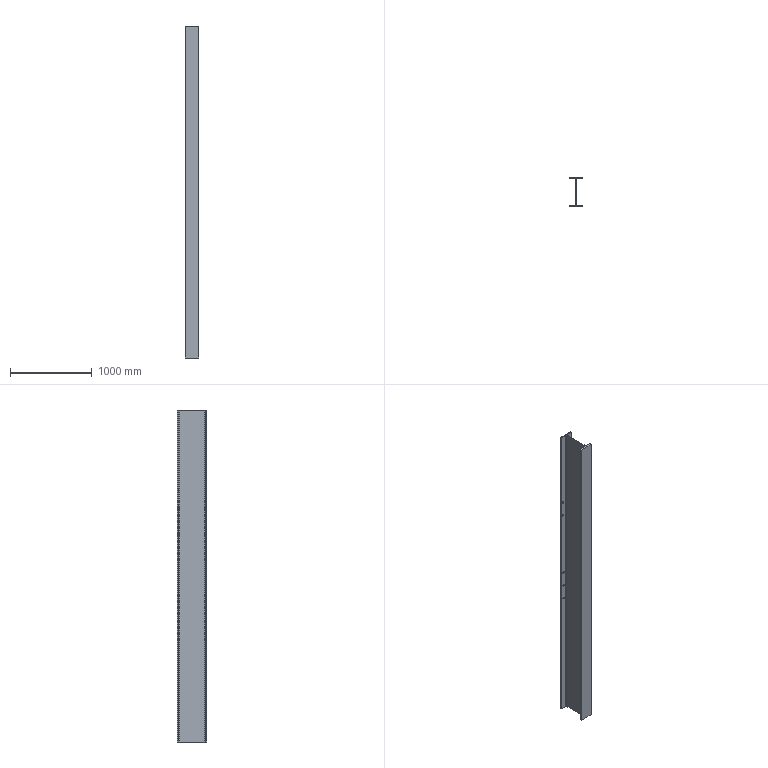Part | SolidWorks | features Chamfer 1, Extrusion 1, ICE 1, SketchHole 1 | 1 solid | 39 faces | box 171.323 x 355.092 x 4064 mm | volume 26304101 mm3 | cylinder 24 | plane 15 | commonest cylinder face diameters 20.574 x20 25.4 x4
STEP:
#1=CARTESIAN_POINT('',(61.087,165.989,1644.65));
#2=VERTEX_POINT('',#1);
#3=CARTESIAN_POINT('',(40.513,165.989,1644.65));
#4=VERTEX_POINT('',#3);
#5=CARTESIAN_POINT('',(50.8,165.989,1644.65));
#6=DIRECTION('',(0.,1.,0.));
#7=DIRECTION('',(-1.,0.,0.));
#8=AXIS2_PLACEMENT_3D('',#5,#6,#7);
#9=CIRCLE('',#8,10.287);
#10=EDGE_CURVE('',#2,#4,#9,.T.);
#11=ORIENTED_EDGE('',*,*,#10,.F.);
#12=CARTESIAN_POINT('',(61.087,177.546,1644.65));
#13=VERTEX_POINT('',#12);
#14=CARTESIAN_POINT('',(61.087,157.546,1644.65));
#15=DIRECTION('',(0.,1.,0.));
#16=VECTOR('',#15,1000.);
#17=LINE('',#14,#16);
#18=EDGE_CURVE('',#2,#13,#17,.T.);
#19=ORIENTED_EDGE('',*,*,#18,.T.);
#20=CARTESIAN_POINT('',(40.513,177.546,1644.65));
#21=VERTEX_POINT('',#20);
#22=CARTESIAN_POINT('',(50.8,177.546,1644.65));
#23=DIRECTION('',(0.,1.,0.));
#24=DIRECTION('',(-1.,0.,0.));
#25=AXIS2_PLACEMENT_3D('',#22,#23,#24);
#26=CIRCLE('',#25,10.287);
#27=EDGE_CURVE('',#13,#21,#26,.T.);
#28=ORIENTED_EDGE('',*,*,#27,.T.);
#29=CARTESIAN_POINT('',(40.513,157.546,1644.65));
#30=DIRECTION('',(0.,1.,0.));
#31=VECTOR('',#30,1000.);
#32=LINE('',#29,#31);
#33=EDGE_CURVE('',#4,#21,#32,.T.);
#34=ORIENTED_EDGE('',*,*,#33,.F.);
#35=EDGE_LOOP('',(#11,#19,#28,#34));
#36=FACE_OUTER_BOUND('',#35,.T.);
#37=CARTESIAN_POINT('',(50.8,157.546,1644.65));
#38=DIRECTION('',(0.,1.,0.));
#39=DIRECTION('',(-1.,0.,0.));
#40=AXIS2_PLACEMENT_3D('',#37,#38,#39);
#41=CYLINDRICAL_SURFACE('',#40,10.287);
#42=ADVANCED_FACE('',(#36),#41,.F.);
#43=CARTESIAN_POINT('',(61.087,165.989,1835.15));
#44=VERTEX_POINT('',#43);
#45=CARTESIAN_POINT('',(40.513,165.989,1835.15));
#46=VERTEX_POINT('',#45);
#47=CARTESIAN_POINT('',(50.8,165.989,1835.15));
#48=DIRECTION('',(0.,1.,0.));
#49=DIRECTION('',(-1.,0.,0.));
#50=AXIS2_PLACEMENT_3D('',#47,#48,#49);
#51=CIRCLE('',#50,10.287);
#52=EDGE_CURVE('',#44,#46,#51,.T.);
#53=ORIENTED_EDGE('',*,*,#52,.F.);
#54=CARTESIAN_POINT('',(61.087,177.546,1835.15));
#55=VERTEX_POINT('',#54);
#56=CARTESIAN_POINT('',(61.087,157.546,1835.15));
#57=DIRECTION('',(0.,1.,0.));
#58=VECTOR('',#57,1000.);
#59=LINE('',#56,#58);
#60=EDGE_CURVE('',#44,#55,#59,.T.);
#61=ORIENTED_EDGE('',*,*,#60,.T.);
#62=CARTESIAN_POINT('',(40.513,177.546,1835.15));
#63=VERTEX_POINT('',#62);
#64=CARTESIAN_POINT('',(50.8,177.546,1835.15));
#65=DIRECTION('',(0.,1.,0.));
#66=DIRECTION('',(-1.,0.,0.));
#67=AXIS2_PLACEMENT_3D('',#64,#65,#66);
#68=CIRCLE('',#67,10.287);
#69=EDGE_CURVE('',#55,#63,#68,.T.);
#70=ORIENTED_EDGE('',*,*,#69,.T.);
#71=CARTESIAN_POINT('',(40.513,157.546,1835.15));
#72=DIRECTION('',(0.,1.,0.));
#73=VECTOR('',#72,1000.);
#74=LINE('',#71,#73);
#75=EDGE_CURVE('',#46,#63,#74,.T.);
#76=ORIENTED_EDGE('',*,*,#75,.F.);
#77=EDGE_LOOP('',(#53,#61,#70,#76));
#78=FACE_OUTER_BOUND('',#77,.T.);
#79=CARTESIAN_POINT('',(50.8,157.546,1835.15));
#80=DIRECTION('',(0.,1.,0.));
#81=DIRECTION('',(-1.,0.,0.));
#82=AXIS2_PLACEMENT_3D('',#79,#80,#81);
#83=CYLINDRICAL_SURFACE('',#82,10.287);
#84=ADVANCED_FACE('',(#78),#83,.F.);
#85=CARTESIAN_POINT('',(-40.513,165.989,1644.65));
#86=VERTEX_POINT('',#85);
#87=CARTESIAN_POINT('',(-61.087,165.989,1644.65));
#88=VERTEX_POINT('',#87);
#89=CARTESIAN_POINT('',(-50.8,165.989,1644.65));
#90=DIRECTION('',(0.,1.,0.));
#91=DIRECTION('',(0.,0.,1.));
#92=AXIS2_PLACEMENT_3D('',#89,#90,#91);
#93=CIRCLE('',#92,10.287);
#94=EDGE_CURVE('',#86,#88,#93,.T.);
#95=ORIENTED_EDGE('',*,*,#94,.F.);
#96=CARTESIAN_POINT('',(-40.513,177.546,1644.65));
#97=VERTEX_POINT('',#96);
#98=CARTESIAN_POINT('',(-40.513,157.546,1644.65));
#99=DIRECTION('',(0.,1.,0.));
#100=VECTOR('',#99,1000.);
#101=LINE('',#98,#100);
#102=EDGE_CURVE('',#86,#97,#101,.T.);
#103=ORIENTED_EDGE('',*,*,#102,.T.);
#104=CARTESIAN_POINT('',(-61.087,177.546,1644.65));
#105=VERTEX_POINT('',#104);
#106=CARTESIAN_POINT('',(-50.8,177.546,1644.65));
#107=DIRECTION('',(0.,1.,0.));
#108=DIRECTION('',(-1.,0.,0.));
#109=AXIS2_PLACEMENT_3D('',#106,#107,#108);
#110=CIRCLE('',#109,10.287);
#111=EDGE_CURVE('',#97,#105,#110,.T.);
#112=ORIENTED_EDGE('',*,*,#111,.T.);
#113=CARTESIAN_POINT('',(-61.087,157.546,1644.65));
#114=DIRECTION('',(0.,1.,0.));
#115=VECTOR('',#114,1000.);
#116=LINE('',#113,#115);
#117=EDGE_CURVE('',#88,#105,#116,.T.);
#118=ORIENTED_EDGE('',*,*,#117,.F.);
#119=EDGE_LOOP('',(#95,#103,#112,#118));
#120=FACE_OUTER_BOUND('',#119,.T.);
#121=CARTESIAN_POINT('',(-50.8,157.546,1644.65));
#122=DIRECTION('',(0.,1.,0.));
#123=DIRECTION('',(-1.,0.,0.));
#124=AXIS2_PLACEMENT_3D('',#121,#122,#123);
#125=CYLINDRICAL_SURFACE('',#124,10.287);
#126=ADVANCED_FACE('',(#120),#125,.F.);
#127=CARTESIAN_POINT('',(-40.513,165.989,1835.15));
#128=VERTEX_POINT('',#127);
#129=CARTESIAN_POINT('',(-61.087,165.989,1835.15));
#130=VERTEX_POINT('',#129);
#131=CARTESIAN_POINT('',(-50.8,165.989,1835.15));
#132=DIRECTION('',(0.,1.,0.));
#133=DIRECTION('',(0.,0.,1.));
#134=AXIS2_PLACEMENT_3D('',#131,#132,#133);
#135=CIRCLE('',#134,10.287);
#136=EDGE_CURVE('',#128,#130,#135,.T.);
#137=ORIENTED_EDGE('',*,*,#136,.F.);
#138=CARTESIAN_POINT('',(-40.513,177.546,1835.15));
#139=VERTEX_POINT('',#138);
#140=CARTESIAN_POINT('',(-40.513,157.546,1835.15));
#141=DIRECTION('',(0.,1.,0.));
#142=VECTOR('',#141,1000.);
#143=LINE('',#140,#142);
#144=EDGE_CURVE('',#128,#139,#143,.T.);
#145=ORIENTED_EDGE('',*,*,#144,.T.);
#146=CARTESIAN_POINT('',(-61.087,177.546,1835.15));
#147=VERTEX_POINT('',#146);
#148=CARTESIAN_POINT('',(-50.8,177.546,1835.15));
#149=DIRECTION('',(0.,1.,0.));
#150=DIRECTION('',(-1.,0.,0.));
#151=AXIS2_PLACEMENT_3D('',#148,#149,#150);
#152=CIRCLE('',#151,10.287);
#153=EDGE_CURVE('',#139,#147,#152,.T.);
#154=ORIENTED_EDGE('',*,*,#153,.T.);
#155=CARTESIAN_POINT('',(-61.087,157.546,1835.15));
#156=DIRECTION('',(0.,1.,0.));
#157=VECTOR('',#156,1000.);
#158=LINE('',#155,#157);
#159=EDGE_CURVE('',#130,#147,#158,.T.);
#160=ORIENTED_EDGE('',*,*,#159,.F.);
#161=EDGE_LOOP('',(#137,#145,#154,#160));
#162=FACE_OUTER_BOUND('',#161,.T.);
#163=CARTESIAN_POINT('',(-50.8,157.546,1835.15));
#164=DIRECTION('',(0.,1.,0.));
#165=DIRECTION('',(-1.,0.,0.));
#166=AXIS2_PLACEMENT_3D('',#163,#164,#165);
#167=CYLINDRICAL_SURFACE('',#166,10.287);
#168=ADVANCED_FACE('',(#162),#167,.F.);
#169=CARTESIAN_POINT('',(-40.513,165.989,2025.65));
#170=VERTEX_POINT('',#169);
#171=CARTESIAN_POINT('',(-61.087,165.989,2025.65));
#172=VERTEX_POINT('',#171);
#173=CARTESIAN_POINT('',(-50.8,165.989,2025.65));
#174=DIRECTION('',(0.,1.,0.));
#175=DIRECTION('',(0.,0.,1.));
#176=AXIS2_PLACEMENT_3D('',#173,#174,#175);
#177=CIRCLE('',#176,10.287);
#178=EDGE_CURVE('',#170,#172,#177,.T.);
#179=ORIENTED_EDGE('',*,*,#178,.F.);
#180=CARTESIAN_POINT('',(-40.513,177.546,2025.65));
#181=VERTEX_POINT('',#180);
#182=CARTESIAN_POINT('',(-40.513,157.546,2025.65));
#183=DIRECTION('',(0.,1.,0.));
#184=VECTOR('',#183,1000.);
#185=LINE('',#182,#184);
#186=EDGE_CURVE('',#170,#181,#185,.T.);
#187=ORIENTED_EDGE('',*,*,#186,.T.);
#188=CARTESIAN_POINT('',(-61.087,177.546,2025.65));
#189=VERTEX_POINT('',#188);
#190=CARTESIAN_POINT('',(-50.8,177.546,2025.65));
#191=DIRECTION('',(0.,1.,0.));
#192=DIRECTION('',(-1.,0.,0.));
#193=AXIS2_PLACEMENT_3D('',#190,#191,#192);
#194=CIRCLE('',#193,10.287);
#195=EDGE_CURVE('',#181,#189,#194,.T.);
#196=ORIENTED_EDGE('',*,*,#195,.T.);
#197=CARTESIAN_POINT('',(-61.087,157.546,2025.65));
#198=DIRECTION('',(0.,1.,0.));
#199=VECTOR('',#198,1000.);
#200=LINE('',#197,#199);
#201=EDGE_CURVE('',#172,#189,#200,.T.);
#202=ORIENTED_EDGE('',*,*,#201,.F.);
#203=EDGE_LOOP('',(#179,#187,#196,#202));
#204=FACE_OUTER_BOUND('',#203,.T.);
#205=CARTESIAN_POINT('',(-50.8,157.546,2025.65));
#206=DIRECTION('',(0.,1.,0.));
#207=DIRECTION('',(-1.,0.,0.));
#208=AXIS2_PLACEMENT_3D('',#205,#206,#207);
#209=CYLINDRICAL_SURFACE('',#208,10.287);
#210=ADVANCED_FACE('',(#204),#209,.F.);
#211=CARTESIAN_POINT('',(61.087,165.989,2025.65));
#212=VERTEX_POINT('',#211);
#213=CARTESIAN_POINT('',(40.513,165.989,2025.65));
#214=VERTEX_POINT('',#213);
#215=CARTESIAN_POINT('',(50.8,165.989,2025.65));
#216=DIRECTION('',(0.,1.,0.));
#217=DIRECTION('',(-1.,0.,0.));
#218=AXIS2_PLACEMENT_3D('',#215,#216,#217);
#219=CIRCLE('',#218,10.287);
#220=EDGE_CURVE('',#212,#214,#219,.T.);
#221=ORIENTED_EDGE('',*,*,#220,.F.);
#222=CARTESIAN_POINT('',(61.087,177.546,2025.65));
#223=VERTEX_POINT('',#222);
#224=CARTESIAN_POINT('',(61.087,157.546,2025.65));
#225=DIRECTION('',(0.,1.,0.));
#226=VECTOR('',#225,1000.);
#227=LINE('',#224,#226);
#228=EDGE_CURVE('',#212,#223,#227,.T.);
#229=ORIENTED_EDGE('',*,*,#228,.T.);
#230=CARTESIAN_POINT('',(40.513,177.546,2025.65));
#231=VERTEX_POINT('',#230);
#232=CARTESIAN_POINT('',(50.8,177.546,2025.65));
#233=DIRECTION('',(0.,1.,0.));
#234=DIRECTION('',(-1.,0.,0.));
#235=AXIS2_PLACEMENT_3D('',#232,#233,#234);
#236=CIRCLE('',#235,10.287);
#237=EDGE_CURVE('',#223,#231,#236,.T.);
#238=ORIENTED_EDGE('',*,*,#237,.T.);
#239=CARTESIAN_POINT('',(40.513,157.546,2025.65));
#240=DIRECTION('',(0.,1.,0.));
#241=VECTOR('',#240,1000.);
#242=LINE('',#239,#241);
#243=EDGE_CURVE('',#214,#231,#242,.T.);
#244=ORIENTED_EDGE('',*,*,#243,.F.);
#245=EDGE_LOOP('',(#221,#229,#238,#244));
#246=FACE_OUTER_BOUND('',#245,.T.);
#247=CARTESIAN_POINT('',(50.8,157.546,2025.65));
#248=DIRECTION('',(0.,1.,0.));
#249=DIRECTION('',(-1.,0.,0.));
#250=AXIS2_PLACEMENT_3D('',#247,#248,#249);
#251=CYLINDRICAL_SURFACE('',#250,10.287);
#252=ADVANCED_FACE('',(#246),#251,.F.);
#253=CARTESIAN_POINT('',(53.213,165.989,2889.25));
#254=VERTEX_POINT('',#253);
#255=CARTESIAN_POINT('',(73.787,165.989,2889.25));
#256=VERTEX_POINT('',#255);
#257=CARTESIAN_POINT('',(63.5,165.989,2889.25));
#258=DIRECTION('',(0.,-1.,0.));
#259=DIRECTION('',(-1.,0.,0.));
#260=AXIS2_PLACEMENT_3D('',#257,#258,#259);
#261=CIRCLE('',#260,10.287);
#262=EDGE_CURVE('',#254,#256,#261,.T.);
#263=ORIENTED_EDGE('',*,*,#262,.T.);
#264=CARTESIAN_POINT('',(73.787,177.546,2889.25));
#265=VERTEX_POINT('',#264);
#266=CARTESIAN_POINT('',(73.787,136.893,2889.25));
#267=DIRECTION('',(0.,1.,0.));
#268=VECTOR('',#267,1000.);
#269=LINE('',#266,#268);
#270=EDGE_CURVE('',#256,#265,#269,.T.);
#271=ORIENTED_EDGE('',*,*,#270,.T.);
#272=CARTESIAN_POINT('',(53.213,177.546,2889.25));
#273=VERTEX_POINT('',#272);
#274=CARTESIAN_POINT('',(63.5,177.546,2889.25));
#275=DIRECTION('',(0.,1.,0.));
#276=DIRECTION('',(-1.,0.,0.));
#277=AXIS2_PLACEMENT_3D('',#274,#275,#276);
#278=CIRCLE('',#277,10.287);
#279=EDGE_CURVE('',#265,#273,#278,.T.);
#280=ORIENTED_EDGE('',*,*,#279,.T.);
#281=CARTESIAN_POINT('',(53.213,136.893,2889.25));
#282=DIRECTION('',(0.,1.,0.));
#283=VECTOR('',#282,1000.);
#284=LINE('',#281,#283);
#285=EDGE_CURVE('',#254,#273,#284,.T.);
#286=ORIENTED_EDGE('',*,*,#285,.F.);
#287=EDGE_LOOP('',(#263,#271,#280,#286));
#288=FACE_OUTER_BOUND('',#287,.T.);
#289=CARTESIAN_POINT('',(63.5,136.893,2889.25));
#290=DIRECTION('',(0.,1.,0.));
#291=DIRECTION('',(-1.,0.,0.));
#292=AXIS2_PLACEMENT_3D('',#289,#290,#291);
#293=CYLINDRICAL_SURFACE('',#292,10.287);
#294=ADVANCED_FACE('',(#288),#293,.F.);
#295=CARTESIAN_POINT('',(-73.787,165.989,2889.25));
#296=VERTEX_POINT('',#295);
#297=CARTESIAN_POINT('',(-53.213,165.989,2889.25));
#298=VERTEX_POINT('',#297);
#299=CARTESIAN_POINT('',(-63.5,165.989,2889.25));
#300=DIRECTION('',(0.,-1.,0.));
#301=DIRECTION('',(-1.,0.,0.));
#302=AXIS2_PLACEMENT_3D('',#299,#300,#301);
#303=CIRCLE('',#302,10.287);
#304=EDGE_CURVE('',#296,#298,#303,.T.);
#305=ORIENTED_EDGE('',*,*,#304,.T.);
#306=CARTESIAN_POINT('',(-53.213,177.546,2889.25));
#307=VERTEX_POINT('',#306);
#308=CARTESIAN_POINT('',(-53.213,136.893,2889.25));
#309=DIRECTION('',(0.,1.,0.));
#310=VECTOR('',#309,1000.);
#311=LINE('',#308,#310);
#312=EDGE_CURVE('',#298,#307,#311,.T.);
#313=ORIENTED_EDGE('',*,*,#312,.T.);
#314=CARTESIAN_POINT('',(-73.787,177.546,2889.25));
#315=VERTEX_POINT('',#314);
#316=CARTESIAN_POINT('',(-63.5,177.546,2889.25));
#317=DIRECTION('',(0.,1.,0.));
#318=DIRECTION('',(-1.,0.,0.));
#319=AXIS2_PLACEMENT_3D('',#316,#317,#318);
#320=CIRCLE('',#319,10.287);
#321=EDGE_CURVE('',#307,#315,#320,.T.);
#322=ORIENTED_EDGE('',*,*,#321,.T.);
#323=CARTESIAN_POINT('',(-73.787,136.893,2889.25));
#324=DIRECTION('',(0.,1.,0.));
#325=VECTOR('',#324,1000.);
#326=LINE('',#323,#325);
#327=EDGE_CURVE('',#296,#315,#326,.T.);
#328=ORIENTED_EDGE('',*,*,#327,.F.);
#329=EDGE_LOOP('',(#305,#313,#322,#328));
#330=FACE_OUTER_BOUND('',#329,.T.);
#331=CARTESIAN_POINT('',(-63.5,136.893,2889.25));
#332=DIRECTION('',(0.,1.,0.));
#333=DIRECTION('',(-1.,0.,0.));
#334=AXIS2_PLACEMENT_3D('',#331,#332,#333);
#335=CYLINDRICAL_SURFACE('',#334,10.287);
#336=ADVANCED_FACE('',(#330),#335,.F.);
#337=CARTESIAN_POINT('',(-73.787,165.989,3079.75));
#338=VERTEX_POINT('',#337);
#339=CARTESIAN_POINT('',(-53.213,165.989,3079.75));
#340=VERTEX_POINT('',#339);
#341=CARTESIAN_POINT('',(-63.5,165.989,3079.75));
#342=DIRECTION('',(0.,-1.,0.));
#343=DIRECTION('',(-1.,0.,0.));
#344=AXIS2_PLACEMENT_3D('',#341,#342,#343);
#345=CIRCLE('',#344,10.287);
#346=EDGE_CURVE('',#338,#340,#345,.T.);
#347=ORIENTED_EDGE('',*,*,#346,.T.);
#348=CARTESIAN_POINT('',(-53.213,177.546,3079.75));
#349=VERTEX_POINT('',#348);
#350=CARTESIAN_POINT('',(-53.213,136.893,3079.75));
#351=DIRECTION('',(0.,1.,0.));
#352=VECTOR('',#351,1000.);
#353=LINE('',#350,#352);
#354=EDGE_CURVE('',#340,#349,#353,.T.);
#355=ORIENTED_EDGE('',*,*,#354,.T.);
#356=CARTESIAN_POINT('',(-73.787,177.546,3079.75));
#357=VERTEX_POINT('',#356);
#358=CARTESIAN_POINT('',(-63.5,177.546,3079.75));
#359=DIRECTION('',(0.,1.,0.));
#360=DIRECTION('',(-1.,0.,0.));
#361=AXIS2_PLACEMENT_3D('',#358,#359,#360);
#362=CIRCLE('',#361,10.287);
#363=EDGE_CURVE('',#349,#357,#362,.T.);
#364=ORIENTED_EDGE('',*,*,#363,.T.);
#365=CARTESIAN_POINT('',(-73.787,136.893,3079.75));
#366=DIRECTION('',(0.,1.,0.));
#367=VECTOR('',#366,1000.);
#368=LINE('',#365,#367);
#369=EDGE_CURVE('',#338,#357,#368,.T.);
#370=ORIENTED_EDGE('',*,*,#369,.F.);
#371=EDGE_LOOP('',(#347,#355,#364,#370));
#372=FACE_OUTER_BOUND('',#371,.T.);
#373=CARTESIAN_POINT('',(-63.5,136.893,3079.75));
#374=DIRECTION('',(0.,1.,0.));
#375=DIRECTION('',(-1.,0.,0.));
#376=AXIS2_PLACEMENT_3D('',#373,#374,#375);
#377=CYLINDRICAL_SURFACE('',#376,10.287);
#378=ADVANCED_FACE('',(#372),#377,.F.);
#379=CARTESIAN_POINT('',(53.213,165.989,3079.75));
#380=VERTEX_POINT('',#379);
#381=CARTESIAN_POINT('',(73.787,165.989,3079.75));
#382=VERTEX_POINT('',#381);
#383=CARTESIAN_POINT('',(63.5,165.989,3079.75));
#384=DIRECTION('',(0.,-1.,0.));
#385=DIRECTION('',(-1.,0.,0.));
#386=AXIS2_PLACEMENT_3D('',#383,#384,#385);
#387=CIRCLE('',#386,10.287);
#388=EDGE_CURVE('',#380,#382,#387,.T.);
#389=ORIENTED_EDGE('',*,*,#388,.T.);
#390=CARTESIAN_POINT('',(73.787,177.546,3079.75));
#391=VERTEX_POINT('',#390);
#392=CARTESIAN_POINT('',(73.787,136.893,3079.75));
#393=DIRECTION('',(0.,1.,0.));
#394=VECTOR('',#393,1000.);
#395=LINE('',#392,#394);
#396=EDGE_CURVE('',#382,#391,#395,.T.);
#397=ORIENTED_EDGE('',*,*,#396,.T.);
#398=CARTESIAN_POINT('',(53.213,177.546,3079.75));
#399=VERTEX_POINT('',#398);
#400=CARTESIAN_POINT('',(63.5,177.546,3079.75));
#401=DIRECTION('',(0.,1.,0.));
#402=DIRECTION('',(-1.,0.,0.));
#403=AXIS2_PLACEMENT_3D('',#400,#401,#402);
#404=CIRCLE('',#403,10.287);
#405=EDGE_CURVE('',#391,#399,#404,.T.);
#406=ORIENTED_EDGE('',*,*,#405,.T.);
#407=CARTESIAN_POINT('',(53.213,136.893,3079.75));
#408=DIRECTION('',(0.,1.,0.));
#409=VECTOR('',#408,1000.);
#410=LINE('',#407,#409);
#411=EDGE_CURVE('',#380,#399,#410,.T.);
#412=ORIENTED_EDGE('',*,*,#411,.F.);
#413=EDGE_LOOP('',(#389,#397,#406,#412));
#414=FACE_OUTER_BOUND('',#413,.T.);
#415=CARTESIAN_POINT('',(63.5,136.893,3079.75));
#416=DIRECTION('',(0.,1.,0.));
#417=DIRECTION('',(-1.,0.,0.));
#418=AXIS2_PLACEMENT_3D('',#415,#416,#417);
#419=CYLINDRICAL_SURFACE('',#418,10.287);
#420=ADVANCED_FACE('',(#414),#419,.F.);
#421=CARTESIAN_POINT('',(-85.661,177.546,0.));
#422=VERTEX_POINT('',#421);
#423=CARTESIAN_POINT('',(-85.661,165.989,0.));
#424=VERTEX_POINT('',#423);
#425=CARTESIAN_POINT('',(-85.661,177.546,0.));
#426=DIRECTION('',(0.,-1.,0.));
#427=VECTOR('',#426,1000.);
#428=LINE('',#425,#427);
#429=EDGE_CURVE('',#422,#424,#428,.T.);
#430=ORIENTED_EDGE('',*,*,#429,.T.);
#431=CARTESIAN_POINT('',(-85.661,165.989,4064.));
#432=VERTEX_POINT('',#431);
#433=CARTESIAN_POINT('',(-85.661,165.989,4064.));
#434=DIRECTION('',(0.,0.,-1.));
#435=VECTOR('',#434,1000.);
#436=LINE('',#433,#435);
#437=EDGE_CURVE('',#432,#424,#436,.T.);
#438=ORIENTED_EDGE('',*,*,#437,.F.);
#439=CARTESIAN_POINT('',(-85.661,177.546,4064.));
#440=VERTEX_POINT('',#439);
#441=CARTESIAN_POINT('',(-85.661,177.546,4064.));
#442=DIRECTION('',(0.,-1.,0.));
#443=VECTOR('',#442,1000.);
#444=LINE('',#441,#443);
#445=EDGE_CURVE('',#440,#432,#444,.T.);
#446=ORIENTED_EDGE('',*,*,#445,.F.);
#447=CARTESIAN_POINT('',(-85.661,177.546,4064.));
#448=DIRECTION('',(0.,0.,-1.));
#449=VECTOR('',#448,1000.);
#450=LINE('',#447,#449);
#451=EDGE_CURVE('',#440,#422,#450,.T.);
#452=ORIENTED_EDGE('',*,*,#451,.T.);
#453=EDGE_LOOP('',(#430,#438,#446,#452));
#454=FACE_OUTER_BOUND('',#453,.T.);
#455=CARTESIAN_POINT('',(-85.661,177.546,4064.));
#456=DIRECTION('',(1.,0.,0.));
#457=DIRECTION('',(0.,0.,-1.));
#458=AXIS2_PLACEMENT_3D('',#455,#456,#457);
#459=PLANE('',#458);
#460=ADVANCED_FACE('',(#454),#459,.F.);
#461=CARTESIAN_POINT('',(-50.8,165.989,1644.65));
#462=DIRECTION('',(0.,1.,0.));
#463=DIRECTION('',(0.,0.,1.));
#464=AXIS2_PLACEMENT_3D('',#461,#462,#463);
#465=CIRCLE('',#464,10.287);
#466=EDGE_CURVE('',#88,#86,#465,.T.);
#467=ORIENTED_EDGE('',*,*,#466,.T.);
#468=ORIENTED_EDGE('',*,*,#94,.T.);
#469=EDGE_LOOP('',(#467,#468));
#470=FACE_BOUND('',#469,.T.);
#471=CARTESIAN_POINT('',(-50.8,165.989,1835.15));
#472=DIRECTION('',(0.,1.,0.));
#473=DIRECTION('',(0.,0.,1.));
#474=AXIS2_PLACEMENT_3D('',#471,#472,#473);
#475=CIRCLE('',#474,10.287);
#476=EDGE_CURVE('',#130,#128,#475,.T.);
#477=ORIENTED_EDGE('',*,*,#476,.T.);
#478=ORIENTED_EDGE('',*,*,#136,.T.);
#479=EDGE_LOOP('',(#477,#478));
#480=FACE_BOUND('',#479,.T.);
#481=CARTESIAN_POINT('',(-50.8,165.989,2025.65));
#482=DIRECTION('',(0.,1.,0.));
#483=DIRECTION('',(0.,0.,1.));
#484=AXIS2_PLACEMENT_3D('',#481,#482,#483);
#485=CIRCLE('',#484,10.287);
#486=EDGE_CURVE('',#172,#170,#485,.T.);
#487=ORIENTED_EDGE('',*,*,#486,.T.);
#488=ORIENTED_EDGE('',*,*,#178,.T.);
#489=EDGE_LOOP('',(#487,#488));
#490=FACE_BOUND('',#489,.T.);
#491=ORIENTED_EDGE('',*,*,#304,.F.);
#492=CARTESIAN_POINT('',(-63.5,165.989,2889.25));
#493=DIRECTION('',(0.,-1.,0.));
#494=DIRECTION('',(-1.,0.,0.));
#495=AXIS2_PLACEMENT_3D('',#492,#493,#494);
#496=CIRCLE('',#495,10.287);
#497=EDGE_CURVE('',#298,#296,#496,.T.);
#498=ORIENTED_EDGE('',*,*,#497,.F.);
#499=EDGE_LOOP('',(#491,#498));
#500=FACE_BOUND('',#499,.T.);
#501=ORIENTED_EDGE('',*,*,#346,.F.);
#502=CARTESIAN_POINT('',(-63.5,165.989,3079.75));
#503=DIRECTION('',(0.,-1.,0.));
#504=DIRECTION('',(-1.,0.,0.));
#505=AXIS2_PLACEMENT_3D('',#502,#503,#504);
#506=CIRCLE('',#505,10.287);
#507=EDGE_CURVE('',#340,#338,#506,.T.);
#508=ORIENTED_EDGE('',*,*,#507,.F.);
#509=EDGE_LOOP('',(#501,#508));
#510=FACE_BOUND('',#509,.T.);
#511=CARTESIAN_POINT('',(-16.294,165.989,0.));
#512=VERTEX_POINT('',#511);
#513=CARTESIAN_POINT('',(-85.661,165.989,0.));
#514=DIRECTION('',(1.,0.,0.));
#515=VECTOR('',#514,1000.);
#516=LINE('',#513,#515);
#517=EDGE_CURVE('',#424,#512,#516,.T.);
#518=ORIENTED_EDGE('',*,*,#517,.T.);
#519=CARTESIAN_POINT('',(-16.294,165.989,4064.));
#520=VERTEX_POINT('',#519);
#521=CARTESIAN_POINT('',(-16.294,165.989,4064.));
#522=DIRECTION('',(0.,0.,-1.));
#523=VECTOR('',#522,1000.);
#524=LINE('',#521,#523);
#525=EDGE_CURVE('',#520,#512,#524,.T.);
#526=ORIENTED_EDGE('',*,*,#525,.F.);
#527=CARTESIAN_POINT('',(-85.661,165.989,4064.));
#528=DIRECTION('',(1.,0.,0.));
#529=VECTOR('',#528,1000.);
#530=LINE('',#527,#529);
#531=EDGE_CURVE('',#432,#520,#530,.T.);
#532=ORIENTED_EDGE('',*,*,#531,.F.);
#533=ORIENTED_EDGE('',*,*,#437,.T.);
#534=EDGE_LOOP('',(#518,#526,#532,#533));
#535=FACE_OUTER_BOUND('',#534,.T.);
#536=CARTESIAN_POINT('',(-85.661,165.989,4064.));
#537=DIRECTION('',(0.,1.,0.));
#538=DIRECTION('',(0.,0.,1.));
#539=AXIS2_PLACEMENT_3D('',#536,#537,#538);
#540=PLANE('',#539);
#541=ADVANCED_FACE('',(#470,#480,#490,#500,#510,#535),#540,.F.);
#542=CARTESIAN_POINT('',(-3.594,153.289,0.));
#543=VERTEX_POINT('',#542);
#544=CARTESIAN_POINT('',(-16.294,153.289,0.));
#545=DIRECTION('',(0.,0.,-1.));
#546=DIRECTION('',(-1.,0.,0.));
#547=AXIS2_PLACEMENT_3D('',#544,#545,#546);
#548=CIRCLE('',#547,12.7);
#549=EDGE_CURVE('',#512,#543,#548,.T.);
#550=ORIENTED_EDGE('',*,*,#549,.T.);
#551=CARTESIAN_POINT('',(-3.594,153.289,4064.));
#552=VERTEX_POINT('',#551);
#553=CARTESIAN_POINT('',(-3.594,153.289,4064.));
#554=DIRECTION('',(0.,0.,-1.));
#555=VECTOR('',#554,1000.);
#556=LINE('',#553,#555);
#557=EDGE_CURVE('',#552,#543,#556,.T.);
#558=ORIENTED_EDGE('',*,*,#557,.F.);
#559=CARTESIAN_POINT('',(-16.294,153.289,4064.));
#560=DIRECTION('',(0.,0.,-1.));
#561=DIRECTION('',(-1.,0.,0.));
#562=AXIS2_PLACEMENT_3D('',#559,#560,#561);
#563=CIRCLE('',#562,12.7);
#564=EDGE_CURVE('',#520,#552,#563,.T.);
#565=ORIENTED_EDGE('',*,*,#564,.F.);
#566=ORIENTED_EDGE('',*,*,#525,.T.);
#567=EDGE_LOOP('',(#550,#558,#565,#566));
#568=FACE_OUTER_BOUND('',#567,.T.);
#569=CARTESIAN_POINT('',(-16.294,153.289,4064.));
#570=DIRECTION('',(0.,0.,-1.));
#571=DIRECTION('',(-1.,0.,0.));
#572=AXIS2_PLACEMENT_3D('',#569,#570,#571);
#573=CYLINDRICAL_SURFACE('',#572,12.7);
#574=ADVANCED_FACE('',(#568),#573,.F.);
#575=CARTESIAN_POINT('',(-3.594,-153.289,0.));
#576=VERTEX_POINT('',#575);
#577=CARTESIAN_POINT('',(-3.594,153.289,0.));
#578=DIRECTION('',(0.,-1.,0.));
#579=VECTOR('',#578,1000.);
#580=LINE('',#577,#579);
#581=EDGE_CURVE('',#543,#576,#580,.T.);
#582=ORIENTED_EDGE('',*,*,#581,.T.);
#583=CARTESIAN_POINT('',(-3.594,-153.289,4064.));
#584=VERTEX_POINT('',#583);
#585=CARTESIAN_POINT('',(-3.594,-153.289,4064.));
#586=DIRECTION('',(0.,0.,-1.));
#587=VECTOR('',#586,1000.);
#588=LINE('',#585,#587);
#589=EDGE_CURVE('',#584,#576,#588,.T.);
#590=ORIENTED_EDGE('',*,*,#589,.F.);
#591=CARTESIAN_POINT('',(-3.594,153.289,4064.));
#592=DIRECTION('',(0.,-1.,0.));
#593=VECTOR('',#592,1000.);
#594=LINE('',#591,#593);
#595=EDGE_CURVE('',#552,#584,#594,.T.);
#596=ORIENTED_EDGE('',*,*,#595,.F.);
#597=ORIENTED_EDGE('',*,*,#557,.T.);
#598=EDGE_LOOP('',(#582,#590,#596,#597));
#599=FACE_OUTER_BOUND('',#598,.T.);
#600=CARTESIAN_POINT('',(-3.594,153.289,4064.));
#601=DIRECTION('',(1.,0.,0.));
#602=DIRECTION('',(0.,1.,0.));
#603=AXIS2_PLACEMENT_3D('',#600,#601,#602);
#604=PLANE('',#603);
#605=ADVANCED_FACE('',(#599),#604,.F.);
#606=CARTESIAN_POINT('',(-16.294,-165.989,4063.997));
#607=VERTEX_POINT('',#606);
#608=CARTESIAN_POINT('',(-16.294,-165.989,0.));
#609=VERTEX_POINT('',#608);
#610=CARTESIAN_POINT('',(-16.294,-165.989,4064.));
#611=DIRECTION('',(0.,0.,-1.));
#612=VECTOR('',#611,1000.);
#613=LINE('',#610,#612);
#614=EDGE_CURVE('',#607,#609,#613,.T.);
#615=ORIENTED_EDGE('',*,*,#614,.F.);
#616=CARTESIAN_POINT('',(-16.018,-165.986,4064.));
#617=VERTEX_POINT('',#616);
#618=CARTESIAN_POINT('',(-16.294,-165.989,4063.997));
#619=CARTESIAN_POINT('',(-16.202,-165.989,4063.997));
#620=CARTESIAN_POINT('',(-16.11,-165.988,4063.998));
#621=CARTESIAN_POINT('',(-16.018,-165.986,4064.));
#622=(BOUNDED_CURVE()B_SPLINE_CURVE(3,(#618,#619,#620,#621),.UNSPECIFIED.,.F.,.T.)B_SPLINE_CURVE_WITH_KNOTS((4,4),(0.,0.02174),.UNSPECIFIED.)CURVE()GEOMETRIC_REPRESENTATION_ITEM()RATIONAL_B_SPLINE_CURVE((1.,1.,1.,1.))REPRESENTATION_ITEM(''));
#623=EDGE_CURVE('',#607,#617,#622,.T.);
#624=ORIENTED_EDGE('',*,*,#623,.T.);
#625=CARTESIAN_POINT('',(-16.294,-153.289,4064.));
#626=DIRECTION('',(0.,0.,-1.));
#627=DIRECTION('',(-1.,0.,0.));
#628=AXIS2_PLACEMENT_3D('',#625,#626,#627);
#629=CIRCLE('',#628,12.7);
#630=EDGE_CURVE('',#584,#617,#629,.T.);
#631=ORIENTED_EDGE('',*,*,#630,.F.);
#632=ORIENTED_EDGE('',*,*,#589,.T.);
#633=CARTESIAN_POINT('',(-16.294,-153.289,0.));
#634=DIRECTION('',(0.,0.,-1.));
#635=DIRECTION('',(-1.,0.,0.));
#636=AXIS2_PLACEMENT_3D('',#633,#634,#635);
#637=CIRCLE('',#636,12.7);
#638=EDGE_CURVE('',#576,#609,#637,.T.);
#639=ORIENTED_EDGE('',*,*,#638,.T.);
#640=EDGE_LOOP('',(#615,#624,#631,#632,#639));
#641=FACE_OUTER_BOUND('',#640,.T.);
#642=CARTESIAN_POINT('',(-16.294,-153.289,4064.));
#643=DIRECTION('',(0.,0.,-1.));
#644=DIRECTION('',(-1.,0.,0.));
#645=AXIS2_PLACEMENT_3D('',#642,#643,#644);
#646=CYLINDRICAL_SURFACE('',#645,12.7);
#647=ADVANCED_FACE('',(#641),#646,.F.);
#648=CARTESIAN_POINT('',(-85.661,-165.989,4063.997));
#649=VERTEX_POINT('',#648);
#650=CARTESIAN_POINT('',(-85.661,-165.989,0.));
#651=VERTEX_POINT('',#650);
#652=CARTESIAN_POINT('',(-85.661,-165.989,4064.));
#653=DIRECTION('',(0.,0.,-1.));
#654=VECTOR('',#653,1000.);
#655=LINE('',#652,#654);
#656=EDGE_CURVE('',#649,#651,#655,.T.);
#657=ORIENTED_EDGE('',*,*,#656,.F.);
#658=CARTESIAN_POINT('',(-16.294,-165.989,4063.997));
#659=DIRECTION('',(1.,0.,0.));
#660=VECTOR('',#659,1000.);
#661=LINE('',#658,#660);
#662=EDGE_CURVE('',#649,#607,#661,.T.);
#663=ORIENTED_EDGE('',*,*,#662,.T.);
#664=ORIENTED_EDGE('',*,*,#614,.T.);
#665=CARTESIAN_POINT('',(-16.294,-165.989,0.));
#666=DIRECTION('',(-1.,0.,0.));
#667=VECTOR('',#666,1000.);
#668=LINE('',#665,#667);
#669=EDGE_CURVE('',#609,#651,#668,.T.);
#670=ORIENTED_EDGE('',*,*,#669,.T.);
#671=EDGE_LOOP('',(#657,#663,#664,#670));
#672=FACE_OUTER_BOUND('',#671,.T.);
#673=CARTESIAN_POINT('',(-16.294,-165.989,4064.));
#674=DIRECTION('',(0.,-1.,0.));
#675=DIRECTION('',(0.,0.,-1.));
#676=AXIS2_PLACEMENT_3D('',#673,#674,#675);
#677=PLANE('',#676);
#678=ADVANCED_FACE('',(#672),#677,.F.);
#679=CARTESIAN_POINT('',(-85.661,-177.546,4052.44));
#680=VERTEX_POINT('',#679);
#681=CARTESIAN_POINT('',(-85.661,-177.546,0.));
#682=VERTEX_POINT('',#681);
#683=CARTESIAN_POINT('',(-85.661,-177.546,4064.));
#684=DIRECTION('',(0.,0.,-1.));
#685=VECTOR('',#684,1000.);
#686=LINE('',#683,#685);
#687=EDGE_CURVE('',#680,#682,#686,.T.);
#688=ORIENTED_EDGE('',*,*,#687,.F.);
#689=CARTESIAN_POINT('',(-85.661,-165.986,4064.));
#690=DIRECTION('',(0.,0.7071,0.7071));
#691=VECTOR('',#690,1000.);
#692=LINE('',#689,#691);
#693=EDGE_CURVE('',#680,#649,#692,.T.);
#694=ORIENTED_EDGE('',*,*,#693,.T.);
#695=ORIENTED_EDGE('',*,*,#656,.T.);
#696=CARTESIAN_POINT('',(-85.661,-165.989,0.));
#697=DIRECTION('',(0.,-1.,0.));
#698=VECTOR('',#697,1000.);
#699=LINE('',#696,#698);
#700=EDGE_CURVE('',#651,#682,#699,.T.);
#701=ORIENTED_EDGE('',*,*,#700,.T.);
#702=EDGE_LOOP('',(#688,#694,#695,#701));
#703=FACE_OUTER_BOUND('',#702,.T.);
#704=CARTESIAN_POINT('',(-85.661,-165.989,4064.));
#705=DIRECTION('',(1.,0.,0.));
#706=DIRECTION('',(0.,0.,-1.));
#707=AXIS2_PLACEMENT_3D('',#704,#705,#706);
#708=PLANE('',#707);
#709=ADVANCED_FACE('',(#703),#708,.F.);
#710=CARTESIAN_POINT('',(85.662,-177.546,4052.44));
#711=VERTEX_POINT('',#710);
#712=CARTESIAN_POINT('',(85.662,-177.546,0.));
#713=VERTEX_POINT('',#712);
#714=CARTESIAN_POINT('',(85.662,-177.546,4064.));
#715=DIRECTION('',(0.,0.,-1.));
#716=VECTOR('',#715,1000.);
#717=LINE('',#714,#716);
#718=EDGE_CURVE('',#711,#713,#717,.T.);
#719=ORIENTED_EDGE('',*,*,#718,.F.);
#720=CARTESIAN_POINT('',(-85.661,-177.546,4052.44));
#721=DIRECTION('',(-1.,0.,0.));
#722=VECTOR('',#721,1000.);
#723=LINE('',#720,#722);
#724=EDGE_CURVE('',#711,#680,#723,.T.);
#725=ORIENTED_EDGE('',*,*,#724,.T.);
#726=ORIENTED_EDGE('',*,*,#687,.T.);
#727=CARTESIAN_POINT('',(-85.661,-177.546,0.));
#728=DIRECTION('',(1.,0.,0.));
#729=VECTOR('',#728,1000.);
#730=LINE('',#727,#729);
#731=EDGE_CURVE('',#682,#713,#730,.T.);
#732=ORIENTED_EDGE('',*,*,#731,.T.);
#733=EDGE_LOOP('',(#719,#725,#726,#732));
#734=FACE_OUTER_BOUND('',#733,.T.);
#735=CARTESIAN_POINT('',(-85.661,-177.546,4064.));
#736=DIRECTION('',(0.,1.,0.));
#737=DIRECTION('',(-1.,0.,0.));
#738=AXIS2_PLACEMENT_3D('',#735,#736,#737);
#739=PLANE('',#738);
#740=ADVANCED_FACE('',(#734),#739,.F.);
#741=CARTESIAN_POINT('',(85.662,-165.989,4063.997));
#742=VERTEX_POINT('',#741);
#743=CARTESIAN_POINT('',(85.662,-165.989,0.));
#744=VERTEX_POINT('',#743);
#745=CARTESIAN_POINT('',(85.662,-165.989,4064.));
#746=DIRECTION('',(0.,0.,-1.));
#747=VECTOR('',#746,1000.);
#748=LINE('',#745,#747);
#749=EDGE_CURVE('',#742,#744,#748,.T.);
#750=ORIENTED_EDGE('',*,*,#749,.F.);
#751=CARTESIAN_POINT('',(85.662,-165.986,4064.));
#752=DIRECTION('',(0.,-0.7071,-0.7071));
#753=VECTOR('',#752,1000.);
#754=LINE('',#751,#753);
#755=EDGE_CURVE('',#742,#711,#754,.T.);
#756=ORIENTED_EDGE('',*,*,#755,.T.);
#757=ORIENTED_EDGE('',*,*,#718,.T.);
#758=CARTESIAN_POINT('',(85.662,-165.989,0.));
#759=DIRECTION('',(0.,1.,0.));
#760=VECTOR('',#759,1000.);
#761=LINE('',#758,#760);
#762=EDGE_CURVE('',#713,#744,#761,.T.);
#763=ORIENTED_EDGE('',*,*,#762,.T.);
#764=EDGE_LOOP('',(#750,#756,#757,#763));
#765=FACE_OUTER_BOUND('',#764,.T.);
#766=CARTESIAN_POINT('',(85.662,-165.989,4064.));
#767=DIRECTION('',(-1.,0.,0.));
#768=DIRECTION('',(0.,-1.,0.));
#769=AXIS2_PLACEMENT_3D('',#766,#767,#768);
#770=PLANE('',#769);
#771=ADVANCED_FACE('',(#765),#770,.F.);
#772=CARTESIAN_POINT('',(16.294,-165.989,4063.997));
#773=VERTEX_POINT('',#772);
#774=CARTESIAN_POINT('',(16.294,-165.989,0.));
#775=VERTEX_POINT('',#774);
#776=CARTESIAN_POINT('',(16.294,-165.989,4064.));
#777=DIRECTION('',(0.,0.,-1.));
#778=VECTOR('',#777,1000.);
#779=LINE('',#776,#778);
#780=EDGE_CURVE('',#773,#775,#779,.T.);
#781=ORIENTED_EDGE('',*,*,#780,.F.);
#782=CARTESIAN_POINT('',(-16.294,-165.989,4063.997));
#783=DIRECTION('',(1.,0.,0.));
#784=VECTOR('',#783,1000.);
#785=LINE('',#782,#784);
#786=EDGE_CURVE('',#773,#742,#785,.T.);
#787=ORIENTED_EDGE('',*,*,#786,.T.);
#788=ORIENTED_EDGE('',*,*,#749,.T.);
#789=CARTESIAN_POINT('',(16.294,-165.989,0.));
#790=DIRECTION('',(-1.,0.,0.));
#791=VECTOR('',#790,1000.);
#792=LINE('',#789,#791);
#793=EDGE_CURVE('',#744,#775,#792,.T.);
#794=ORIENTED_EDGE('',*,*,#793,.T.);
#795=EDGE_LOOP('',(#781,#787,#788,#794));
#796=FACE_OUTER_BOUND('',#795,.T.);
#797=CARTESIAN_POINT('',(16.294,-165.989,4064.));
#798=DIRECTION('',(0.,-1.,0.));
#799=DIRECTION('',(0.,0.,-1.));
#800=AXIS2_PLACEMENT_3D('',#797,#798,#799);
#801=PLANE('',#800);
#802=ADVANCED_FACE('',(#796),#801,.F.);
#803=CARTESIAN_POINT('',(16.018,-165.986,4064.));
#804=VERTEX_POINT('',#803);
#805=CARTESIAN_POINT('',(3.594,-153.289,4064.));
#806=VERTEX_POINT('',#805);
#807=CARTESIAN_POINT('',(16.294,-153.289,4064.));
#808=DIRECTION('',(0.,0.,-1.));
#809=DIRECTION('',(1.,0.,0.));
#810=AXIS2_PLACEMENT_3D('',#807,#808,#809);
#811=CIRCLE('',#810,12.7);
#812=EDGE_CURVE('',#804,#806,#811,.T.);
#813=ORIENTED_EDGE('',*,*,#812,.F.);
#814=CARTESIAN_POINT('',(16.018,-165.986,4064.));
#815=CARTESIAN_POINT('',(16.11,-165.988,4063.998));
#816=CARTESIAN_POINT('',(16.202,-165.989,4063.997));
#817=CARTESIAN_POINT('',(16.294,-165.989,4063.997));
#818=(BOUNDED_CURVE()B_SPLINE_CURVE(3,(#814,#815,#816,#817),.UNSPECIFIED.,.F.,.T.)B_SPLINE_CURVE_WITH_KNOTS((4,4),(6.261,6.283),.UNSPECIFIED.)CURVE()GEOMETRIC_REPRESENTATION_ITEM()RATIONAL_B_SPLINE_CURVE((1.,1.,1.,1.))REPRESENTATION_ITEM(''));
#819=EDGE_CURVE('',#804,#773,#818,.T.);
#820=ORIENTED_EDGE('',*,*,#819,.T.);
#821=ORIENTED_EDGE('',*,*,#780,.T.);
#822=CARTESIAN_POINT('',(3.594,-153.289,0.));
#823=VERTEX_POINT('',#822);
#824=CARTESIAN_POINT('',(16.294,-153.289,0.));
#825=DIRECTION('',(0.,0.,-1.));
#826=DIRECTION('',(1.,0.,0.));
#827=AXIS2_PLACEMENT_3D('',#824,#825,#826);
#828=CIRCLE('',#827,12.7);
#829=EDGE_CURVE('',#775,#823,#828,.T.);
#830=ORIENTED_EDGE('',*,*,#829,.T.);
#831=CARTESIAN_POINT('',(3.594,-153.289,4064.));
#832=DIRECTION('',(0.,0.,-1.));
#833=VECTOR('',#832,1000.);
#834=LINE('',#831,#833);
#835=EDGE_CURVE('',#806,#823,#834,.T.);
#836=ORIENTED_EDGE('',*,*,#835,.F.);
#837=EDGE_LOOP('',(#813,#820,#821,#830,#836));
#838=FACE_OUTER_BOUND('',#837,.T.);
#839=CARTESIAN_POINT('',(16.294,-153.289,4064.));
#840=DIRECTION('',(0.,0.,-1.));
#841=DIRECTION('',(-1.,0.,0.));
#842=AXIS2_PLACEMENT_3D('',#839,#840,#841);
#843=CYLINDRICAL_SURFACE('',#842,12.7);
#844=ADVANCED_FACE('',(#838),#843,.F.);
#845=CARTESIAN_POINT('',(3.594,153.289,0.));
#846=VERTEX_POINT('',#845);
#847=CARTESIAN_POINT('',(3.594,153.289,0.));
#848=DIRECTION('',(0.,1.,0.));
#849=VECTOR('',#848,1000.);
#850=LINE('',#847,#849);
#851=EDGE_CURVE('',#823,#846,#850,.T.);
#852=ORIENTED_EDGE('',*,*,#851,.T.);
#853=CARTESIAN_POINT('',(3.594,153.289,4064.));
#854=VERTEX_POINT('',#853);
#855=CARTESIAN_POINT('',(3.594,153.289,4064.));
#856=DIRECTION('',(0.,0.,-1.));
#857=VECTOR('',#856,1000.);
#858=LINE('',#855,#857);
#859=EDGE_CURVE('',#854,#846,#858,.T.);
#860=ORIENTED_EDGE('',*,*,#859,.F.);
#861=CARTESIAN_POINT('',(3.594,153.289,4064.));
#862=DIRECTION('',(0.,1.,0.));
#863=VECTOR('',#862,1000.);
#864=LINE('',#861,#863);
#865=EDGE_CURVE('',#806,#854,#864,.T.);
#866=ORIENTED_EDGE('',*,*,#865,.F.);
#867=ORIENTED_EDGE('',*,*,#835,.T.);
#868=EDGE_LOOP('',(#852,#860,#866,#867));
#869=FACE_OUTER_BOUND('',#868,.T.);
#870=CARTESIAN_POINT('',(3.594,153.289,4064.));
#871=DIRECTION('',(-1.,0.,0.));
#872=DIRECTION('',(0.,-1.,0.));
#873=AXIS2_PLACEMENT_3D('',#870,#871,#872);
#874=PLANE('',#873);
#875=ADVANCED_FACE('',(#869),#874,.F.);
#876=CARTESIAN_POINT('',(16.294,165.989,0.));
#877=VERTEX_POINT('',#876);
#878=CARTESIAN_POINT('',(16.294,153.289,0.));
#879=DIRECTION('',(0.,0.,-1.));
#880=DIRECTION('',(1.,0.,0.));
#881=AXIS2_PLACEMENT_3D('',#878,#879,#880);
#882=CIRCLE('',#881,12.7);
#883=EDGE_CURVE('',#846,#877,#882,.T.);
#884=ORIENTED_EDGE('',*,*,#883,.T.);
#885=CARTESIAN_POINT('',(16.294,165.989,4064.));
#886=VERTEX_POINT('',#885);
#887=CARTESIAN_POINT('',(16.294,165.989,4064.));
#888=DIRECTION('',(0.,0.,-1.));
#889=VECTOR('',#888,1000.);
#890=LINE('',#887,#889);
#891=EDGE_CURVE('',#886,#877,#890,.T.);
#892=ORIENTED_EDGE('',*,*,#891,.F.);
#893=CARTESIAN_POINT('',(16.294,153.289,4064.));
#894=DIRECTION('',(0.,0.,-1.));
#895=DIRECTION('',(1.,0.,0.));
#896=AXIS2_PLACEMENT_3D('',#893,#894,#895);
#897=CIRCLE('',#896,12.7);
#898=EDGE_CURVE('',#854,#886,#897,.T.);
#899=ORIENTED_EDGE('',*,*,#898,.F.);
#900=ORIENTED_EDGE('',*,*,#859,.T.);
#901=EDGE_LOOP('',(#884,#892,#899,#900));
#902=FACE_OUTER_BOUND('',#901,.T.);
#903=CARTESIAN_POINT('',(16.294,153.289,4064.));
#904=DIRECTION('',(0.,0.,-1.));
#905=DIRECTION('',(-1.,0.,0.));
#906=AXIS2_PLACEMENT_3D('',#903,#904,#905);
#907=CYLINDRICAL_SURFACE('',#906,12.7);
#908=ADVANCED_FACE('',(#902),#907,.F.);
#909=CARTESIAN_POINT('',(50.8,165.989,1644.65));
#910=DIRECTION('',(0.,1.,0.));
#911=DIRECTION('',(-1.,0.,0.));
#912=AXIS2_PLACEMENT_3D('',#909,#910,#911);
#913=CIRCLE('',#912,10.287);
#914=EDGE_CURVE('',#4,#2,#913,.T.);
#915=ORIENTED_EDGE('',*,*,#914,.T.);
#916=ORIENTED_EDGE('',*,*,#10,.T.);
#917=EDGE_LOOP('',(#915,#916));
#918=FACE_BOUND('',#917,.T.);
#919=CARTESIAN_POINT('',(50.8,165.989,1835.15));
#920=DIRECTION('',(0.,1.,0.));
#921=DIRECTION('',(-1.,0.,0.));
#922=AXIS2_PLACEMENT_3D('',#919,#920,#921);
#923=CIRCLE('',#922,10.287);
#924=EDGE_CURVE('',#46,#44,#923,.T.);
#925=ORIENTED_EDGE('',*,*,#924,.T.);
#926=ORIENTED_EDGE('',*,*,#52,.T.);
#927=EDGE_LOOP('',(#925,#926));
#928=FACE_BOUND('',#927,.T.);
#929=CARTESIAN_POINT('',(50.8,165.989,2025.65));
#930=DIRECTION('',(0.,1.,0.));
#931=DIRECTION('',(-1.,0.,0.));
#932=AXIS2_PLACEMENT_3D('',#929,#930,#931);
#933=CIRCLE('',#932,10.287);
#934=EDGE_CURVE('',#214,#212,#933,.T.);
#935=ORIENTED_EDGE('',*,*,#934,.T.);
#936=ORIENTED_EDGE('',*,*,#220,.T.);
#937=EDGE_LOOP('',(#935,#936));
#938=FACE_BOUND('',#937,.T.);
#939=ORIENTED_EDGE('',*,*,#262,.F.);
#940=CARTESIAN_POINT('',(63.5,165.989,2889.25));
#941=DIRECTION('',(0.,-1.,0.));
#942=DIRECTION('',(-1.,0.,0.));
#943=AXIS2_PLACEMENT_3D('',#940,#941,#942);
#944=CIRCLE('',#943,10.287);
#945=EDGE_CURVE('',#256,#254,#944,.T.);
#946=ORIENTED_EDGE('',*,*,#945,.F.);
#947=EDGE_LOOP('',(#939,#946));
#948=FACE_BOUND('',#947,.T.);
#949=ORIENTED_EDGE('',*,*,#388,.F.);
#950=CARTESIAN_POINT('',(63.5,165.989,3079.75));
#951=DIRECTION('',(0.,-1.,0.));
#952=DIRECTION('',(-1.,0.,0.));
#953=AXIS2_PLACEMENT_3D('',#950,#951,#952);
#954=CIRCLE('',#953,10.287);
#955=EDGE_CURVE('',#382,#380,#954,.T.);
#956=ORIENTED_EDGE('',*,*,#955,.F.);
#957=EDGE_LOOP('',(#949,#956));
#958=FACE_BOUND('',#957,.T.);
#959=CARTESIAN_POINT('',(85.662,165.989,0.));
#960=VERTEX_POINT('',#959);
#961=CARTESIAN_POINT('',(85.662,165.989,0.));
#962=DIRECTION('',(1.,0.,0.));
#963=VECTOR('',#962,1000.);
#964=LINE('',#961,#963);
#965=EDGE_CURVE('',#877,#960,#964,.T.);
#966=ORIENTED_EDGE('',*,*,#965,.T.);
#967=CARTESIAN_POINT('',(85.662,165.989,4064.));
#968=VERTEX_POINT('',#967);
#969=CARTESIAN_POINT('',(85.662,165.989,4064.));
#970=DIRECTION('',(0.,0.,-1.));
#971=VECTOR('',#970,1000.);
#972=LINE('',#969,#971);
#973=EDGE_CURVE('',#968,#960,#972,.T.);
#974=ORIENTED_EDGE('',*,*,#973,.F.);
#975=CARTESIAN_POINT('',(85.662,165.989,4064.));
#976=DIRECTION('',(1.,0.,0.));
#977=VECTOR('',#976,1000.);
#978=LINE('',#975,#977);
#979=EDGE_CURVE('',#886,#968,#978,.T.);
#980=ORIENTED_EDGE('',*,*,#979,.F.);
#981=ORIENTED_EDGE('',*,*,#891,.T.);
#982=EDGE_LOOP('',(#966,#974,#980,#981));
#983=FACE_OUTER_BOUND('',#982,.T.);
#984=CARTESIAN_POINT('',(85.662,165.989,4064.));
#985=DIRECTION('',(0.,1.,0.));
#986=DIRECTION('',(-1.,0.,0.));
#987=AXIS2_PLACEMENT_3D('',#984,#985,#986);
#988=PLANE('',#987);
#989=ADVANCED_FACE('',(#918,#928,#938,#948,#958,#983),#988,.F.);
#990=CARTESIAN_POINT('',(85.662,177.546,0.));
#991=VERTEX_POINT('',#990);
#992=CARTESIAN_POINT('',(85.662,177.546,0.));
#993=DIRECTION('',(0.,1.,0.));
#994=VECTOR('',#993,1000.);
#995=LINE('',#992,#994);
#996=EDGE_CURVE('',#960,#991,#995,.T.);
#997=ORIENTED_EDGE('',*,*,#996,.T.);
#998=CARTESIAN_POINT('',(85.662,177.546,4064.));
#999=VERTEX_POINT('',#998);
#1000=CARTESIAN_POINT('',(85.662,177.546,4064.));
#1001=DIRECTION('',(0.,0.,-1.));
#1002=VECTOR('',#1001,1000.);
#1003=LINE('',#1000,#1002);
#1004=EDGE_CURVE('',#999,#991,#1003,.T.);
#1005=ORIENTED_EDGE('',*,*,#1004,.F.);
#1006=CARTESIAN_POINT('',(85.662,177.546,4064.));
#1007=DIRECTION('',(0.,1.,0.));
#1008=VECTOR('',#1007,1000.);
#1009=LINE('',#1006,#1008);
#1010=EDGE_CURVE('',#968,#999,#1009,.T.);
#1011=ORIENTED_EDGE('',*,*,#1010,.F.);
#1012=ORIENTED_EDGE('',*,*,#973,.T.);
#1013=EDGE_LOOP('',(#997,#1005,#1011,#1012));
#1014=FACE_OUTER_BOUND('',#1013,.T.);
#1015=CARTESIAN_POINT('',(85.662,177.546,4064.));
#1016=DIRECTION('',(-1.,0.,0.));
#1017=DIRECTION('',(0.,-1.,0.));
#1018=AXIS2_PLACEMENT_3D('',#1015,#1016,#1017);
#1019=PLANE('',#1018);
#1020=ADVANCED_FACE('',(#1014),#1019,.F.);
#1021=CARTESIAN_POINT('',(50.8,177.546,1644.65));
#1022=DIRECTION('',(0.,1.,0.));
#1023=DIRECTION('',(-1.,0.,0.));
#1024=AXIS2_PLACEMENT_3D('',#1021,#1022,#1023);
#1025=CIRCLE('',#1024,10.287);
#1026=EDGE_CURVE('',#21,#13,#1025,.T.);
#1027=ORIENTED_EDGE('',*,*,#1026,.F.);
#1028=ORIENTED_EDGE('',*,*,#27,.F.);
#1029=EDGE_LOOP('',(#1027,#1028));
#1030=FACE_BOUND('',#1029,.T.);
#1031=CARTESIAN_POINT('',(50.8,177.546,1835.15));
#1032=DIRECTION('',(0.,1.,0.));
#1033=DIRECTION('',(-1.,0.,0.));
#1034=AXIS2_PLACEMENT_3D('',#1031,#1032,#1033);
#1035=CIRCLE('',#1034,10.287);
#1036=EDGE_CURVE('',#63,#55,#1035,.T.);
#1037=ORIENTED_EDGE('',*,*,#1036,.F.);
#1038=ORIENTED_EDGE('',*,*,#69,.F.);
#1039=EDGE_LOOP('',(#1037,#1038));
#1040=FACE_BOUND('',#1039,.T.);
#1041=CARTESIAN_POINT('',(-50.8,177.546,1644.65));
#1042=DIRECTION('',(0.,1.,0.));
#1043=DIRECTION('',(-1.,0.,0.));
#1044=AXIS2_PLACEMENT_3D('',#1041,#1042,#1043);
#1045=CIRCLE('',#1044,10.287);
#1046=EDGE_CURVE('',#105,#97,#1045,.T.);
#1047=ORIENTED_EDGE('',*,*,#1046,.F.);
#1048=ORIENTED_EDGE('',*,*,#111,.F.);
#1049=EDGE_LOOP('',(#1047,#1048));
#1050=FACE_BOUND('',#1049,.T.);
#1051=CARTESIAN_POINT('',(-50.8,177.546,1835.15));
#1052=DIRECTION('',(0.,1.,0.));
#1053=DIRECTION('',(-1.,0.,0.));
#1054=AXIS2_PLACEMENT_3D('',#1051,#1052,#1053);
#1055=CIRCLE('',#1054,10.287);
#1056=EDGE_CURVE('',#147,#139,#1055,.T.);
#1057=ORIENTED_EDGE('',*,*,#1056,.F.);
#1058=ORIENTED_EDGE('',*,*,#153,.F.);
#1059=EDGE_LOOP('',(#1057,#1058));
#1060=FACE_BOUND('',#1059,.T.);
#1061=CARTESIAN_POINT('',(-50.8,177.546,2025.65));
#1062=DIRECTION('',(0.,1.,0.));
#1063=DIRECTION('',(-1.,0.,0.));
#1064=AXIS2_PLACEMENT_3D('',#1061,#1062,#1063);
#1065=CIRCLE('',#1064,10.287);
#1066=EDGE_CURVE('',#189,#181,#1065,.T.);
#1067=ORIENTED_EDGE('',*,*,#1066,.F.);
#1068=ORIENTED_EDGE('',*,*,#195,.F.);
#1069=EDGE_LOOP('',(#1067,#1068));
#1070=FACE_BOUND('',#1069,.T.);
#1071=CARTESIAN_POINT('',(50.8,177.546,2025.65));
#1072=DIRECTION('',(0.,1.,0.));
#1073=DIRECTION('',(-1.,0.,0.));
#1074=AXIS2_PLACEMENT_3D('',#1071,#1072,#1073);
#1075=CIRCLE('',#1074,10.287);
#1076=EDGE_CURVE('',#231,#223,#1075,.T.);
#1077=ORIENTED_EDGE('',*,*,#1076,.F.);
#1078=ORIENTED_EDGE('',*,*,#237,.F.);
#1079=EDGE_LOOP('',(#1077,#1078));
#1080=FACE_BOUND('',#1079,.T.);
#1081=CARTESIAN_POINT('',(63.5,177.546,2889.25));
#1082=DIRECTION('',(0.,1.,0.));
#1083=DIRECTION('',(-1.,0.,0.));
#1084=AXIS2_PLACEMENT_3D('',#1081,#1082,#1083);
#1085=CIRCLE('',#1084,10.287);
#1086=EDGE_CURVE('',#273,#265,#1085,.T.);
#1087=ORIENTED_EDGE('',*,*,#1086,.F.);
#1088=ORIENTED_EDGE('',*,*,#279,.F.);
#1089=EDGE_LOOP('',(#1087,#1088));
#1090=FACE_BOUND('',#1089,.T.);
#1091=CARTESIAN_POINT('',(-63.5,177.546,2889.25));
#1092=DIRECTION('',(0.,1.,0.));
#1093=DIRECTION('',(-1.,0.,0.));
#1094=AXIS2_PLACEMENT_3D('',#1091,#1092,#1093);
#1095=CIRCLE('',#1094,10.287);
#1096=EDGE_CURVE('',#315,#307,#1095,.T.);
#1097=ORIENTED_EDGE('',*,*,#1096,.F.);
#1098=ORIENTED_EDGE('',*,*,#321,.F.);
#1099=EDGE_LOOP('',(#1097,#1098));
#1100=FACE_BOUND('',#1099,.T.);
#1101=CARTESIAN_POINT('',(-63.5,177.546,3079.75));
#1102=DIRECTION('',(0.,1.,0.));
#1103=DIRECTION('',(-1.,0.,0.));
#1104=AXIS2_PLACEMENT_3D('',#1101,#1102,#1103);
#1105=CIRCLE('',#1104,10.287);
#1106=EDGE_CURVE('',#357,#349,#1105,.T.);
#1107=ORIENTED_EDGE('',*,*,#1106,.F.);
#1108=ORIENTED_EDGE('',*,*,#363,.F.);
#1109=EDGE_LOOP('',(#1107,#1108));
#1110=FACE_BOUND('',#1109,.T.);
#1111=CARTESIAN_POINT('',(63.5,177.546,3079.75));
#1112=DIRECTION('',(0.,1.,0.));
#1113=DIRECTION('',(-1.,0.,0.));
#1114=AXIS2_PLACEMENT_3D('',#1111,#1112,#1113);
#1115=CIRCLE('',#1114,10.287);
#1116=EDGE_CURVE('',#399,#391,#1115,.T.);
#1117=ORIENTED_EDGE('',*,*,#1116,.F.);
#1118=ORIENTED_EDGE('',*,*,#405,.F.);
#1119=EDGE_LOOP('',(#1117,#1118));
#1120=FACE_BOUND('',#1119,.T.);
#1121=CARTESIAN_POINT('',(85.662,177.546,0.));
#1122=DIRECTION('',(-1.,0.,0.));
#1123=VECTOR('',#1122,1000.);
#1124=LINE('',#1121,#1123);
#1125=EDGE_CURVE('',#991,#422,#1124,.T.);
#1126=ORIENTED_EDGE('',*,*,#1125,.T.);
#1127=ORIENTED_EDGE('',*,*,#451,.F.);
#1128=CARTESIAN_POINT('',(85.662,177.546,4064.));
#1129=DIRECTION('',(-1.,0.,0.));
#1130=VECTOR('',#1129,1000.);
#1131=LINE('',#1128,#1130);
#1132=EDGE_CURVE('',#999,#440,#1131,.T.);
#1133=ORIENTED_EDGE('',*,*,#1132,.F.);
#1134=ORIENTED_EDGE('',*,*,#1004,.T.);
#1135=EDGE_LOOP('',(#1126,#1127,#1133,#1134));
#1136=FACE_OUTER_BOUND('',#1135,.T.);
#1137=CARTESIAN_POINT('',(85.662,177.546,4064.));
#1138=DIRECTION('',(0.,-1.,0.));
#1139=DIRECTION('',(1.,0.,0.));
#1140=AXIS2_PLACEMENT_3D('',#1137,#1138,#1139);
#1141=PLANE('',#1140);
#1142=ADVANCED_FACE('',(#1030,#1040,#1050,#1060,#1070,#1080,#1090,#1100,#1110,#1120,#1136),#1141,.F.);
#1143=ORIENTED_EDGE('',*,*,#630,.T.);
#1144=CARTESIAN_POINT('',(-16.294,-165.986,4064.));
#1145=DIRECTION('',(1.,0.,0.));
#1146=VECTOR('',#1145,1000.);
#1147=LINE('',#1144,#1146);
#1148=EDGE_CURVE('',#617,#804,#1147,.T.);
#1149=ORIENTED_EDGE('',*,*,#1148,.T.);
#1150=ORIENTED_EDGE('',*,*,#812,.T.);
#1151=ORIENTED_EDGE('',*,*,#865,.T.);
#1152=ORIENTED_EDGE('',*,*,#898,.T.);
#1153=ORIENTED_EDGE('',*,*,#979,.T.);
#1154=ORIENTED_EDGE('',*,*,#1010,.T.);
#1155=ORIENTED_EDGE('',*,*,#1132,.T.);
#1156=ORIENTED_EDGE('',*,*,#445,.T.);
#1157=ORIENTED_EDGE('',*,*,#531,.T.);
#1158=ORIENTED_EDGE('',*,*,#564,.T.);
#1159=ORIENTED_EDGE('',*,*,#595,.T.);
#1160=EDGE_LOOP('',(#1143,#1149,#1150,#1151,#1152,#1153,#1154,#1155,#1156,#1157,#1158,#1159));
#1161=FACE_OUTER_BOUND('',#1160,.T.);
#1162=CARTESIAN_POINT('',(-16.294,153.289,4064.));
#1163=DIRECTION('',(0.,0.,-1.));
#1164=DIRECTION('',(-1.,0.,0.));
#1165=AXIS2_PLACEMENT_3D('',#1162,#1163,#1164);
#1166=PLANE('',#1165);
#1167=ADVANCED_FACE('',(#1161),#1166,.F.);
#1168=ORIENTED_EDGE('',*,*,#429,.F.);
#1169=ORIENTED_EDGE('',*,*,#1125,.F.);
#1170=ORIENTED_EDGE('',*,*,#996,.F.);
#1171=ORIENTED_EDGE('',*,*,#965,.F.);
#1172=ORIENTED_EDGE('',*,*,#883,.F.);
#1173=ORIENTED_EDGE('',*,*,#851,.F.);
#1174=ORIENTED_EDGE('',*,*,#829,.F.);
#1175=ORIENTED_EDGE('',*,*,#793,.F.);
#1176=ORIENTED_EDGE('',*,*,#762,.F.);
#1177=ORIENTED_EDGE('',*,*,#731,.F.);
#1178=ORIENTED_EDGE('',*,*,#700,.F.);
#1179=ORIENTED_EDGE('',*,*,#669,.F.);
#1180=ORIENTED_EDGE('',*,*,#638,.F.);
#1181=ORIENTED_EDGE('',*,*,#581,.F.);
#1182=ORIENTED_EDGE('',*,*,#549,.F.);
#1183=ORIENTED_EDGE('',*,*,#517,.F.);
#1184=EDGE_LOOP('',(#1168,#1169,#1170,#1171,#1172,#1173,#1174,#1175,#1176,#1177,#1178,#1179,#1180,#1181,#1182,#1183));
#1185=FACE_OUTER_BOUND('',#1184,.T.);
#1186=CARTESIAN_POINT('',(-16.294,153.289,0.));
#1187=DIRECTION('',(0.,0.,-1.));
#1188=DIRECTION('',(-1.,0.,0.));
#1189=AXIS2_PLACEMENT_3D('',#1186,#1187,#1188);
#1190=PLANE('',#1189);
#1191=ADVANCED_FACE('',(#1185),#1190,.T.);
#1192=ORIENTED_EDGE('',*,*,#396,.F.);
#1193=ORIENTED_EDGE('',*,*,#955,.T.);
#1194=ORIENTED_EDGE('',*,*,#411,.T.);
#1195=ORIENTED_EDGE('',*,*,#1116,.T.);
#1196=EDGE_LOOP('',(#1192,#1193,#1194,#1195));
#1197=FACE_OUTER_BOUND('',#1196,.T.);
#1198=CARTESIAN_POINT('',(63.5,136.893,3079.75));
#1199=DIRECTION('',(0.,1.,0.));
#1200=DIRECTION('',(-1.,0.,0.));
#1201=AXIS2_PLACEMENT_3D('',#1198,#1199,#1200);
#1202=CYLINDRICAL_SURFACE('',#1201,10.287);
#1203=ADVANCED_FACE('',(#1197),#1202,.F.);
#1204=ORIENTED_EDGE('',*,*,#354,.F.);
#1205=ORIENTED_EDGE('',*,*,#507,.T.);
#1206=ORIENTED_EDGE('',*,*,#369,.T.);
#1207=ORIENTED_EDGE('',*,*,#1106,.T.);
#1208=EDGE_LOOP('',(#1204,#1205,#1206,#1207));
#1209=FACE_OUTER_BOUND('',#1208,.T.);
#1210=CARTESIAN_POINT('',(-63.5,136.893,3079.75));
#1211=DIRECTION('',(0.,1.,0.));
#1212=DIRECTION('',(-1.,0.,0.));
#1213=AXIS2_PLACEMENT_3D('',#1210,#1211,#1212);
#1214=CYLINDRICAL_SURFACE('',#1213,10.287);
#1215=ADVANCED_FACE('',(#1209),#1214,.F.);
#1216=ORIENTED_EDGE('',*,*,#312,.F.);
#1217=ORIENTED_EDGE('',*,*,#497,.T.);
#1218=ORIENTED_EDGE('',*,*,#327,.T.);
#1219=ORIENTED_EDGE('',*,*,#1096,.T.);
#1220=EDGE_LOOP('',(#1216,#1217,#1218,#1219));
#1221=FACE_OUTER_BOUND('',#1220,.T.);
#1222=CARTESIAN_POINT('',(-63.5,136.893,2889.25));
#1223=DIRECTION('',(0.,1.,0.));
#1224=DIRECTION('',(-1.,0.,0.));
#1225=AXIS2_PLACEMENT_3D('',#1222,#1223,#1224);
#1226=CYLINDRICAL_SURFACE('',#1225,10.287);
#1227=ADVANCED_FACE('',(#1221),#1226,.F.);
#1228=ORIENTED_EDGE('',*,*,#270,.F.);
#1229=ORIENTED_EDGE('',*,*,#945,.T.);
#1230=ORIENTED_EDGE('',*,*,#285,.T.);
#1231=ORIENTED_EDGE('',*,*,#1086,.T.);
#1232=EDGE_LOOP('',(#1228,#1229,#1230,#1231));
#1233=FACE_OUTER_BOUND('',#1232,.T.);
#1234=CARTESIAN_POINT('',(63.5,136.893,2889.25));
#1235=DIRECTION('',(0.,1.,0.));
#1236=DIRECTION('',(-1.,0.,0.));
#1237=AXIS2_PLACEMENT_3D('',#1234,#1235,#1236);
#1238=CYLINDRICAL_SURFACE('',#1237,10.287);
#1239=ADVANCED_FACE('',(#1233),#1238,.F.);
#1240=ORIENTED_EDGE('',*,*,#693,.F.);
#1241=ORIENTED_EDGE('',*,*,#724,.F.);
#1242=ORIENTED_EDGE('',*,*,#755,.F.);
#1243=ORIENTED_EDGE('',*,*,#786,.F.);
#1244=ORIENTED_EDGE('',*,*,#819,.F.);
#1245=ORIENTED_EDGE('',*,*,#1148,.F.);
#1246=ORIENTED_EDGE('',*,*,#623,.F.);
#1247=ORIENTED_EDGE('',*,*,#662,.F.);
#1248=EDGE_LOOP('',(#1240,#1241,#1242,#1243,#1244,#1245,#1246,#1247));
#1249=FACE_OUTER_BOUND('',#1248,.T.);
#1250=CARTESIAN_POINT('',(-16.294,-165.986,4064.));
#1251=DIRECTION('',(0.,0.7071,-0.7071));
#1252=DIRECTION('',(0.,0.7071,0.7071));
#1253=AXIS2_PLACEMENT_3D('',#1250,#1251,#1252);
#1254=PLANE('',#1253);
#1255=ADVANCED_FACE('',(#1249),#1254,.F.);
#1256=ORIENTED_EDGE('',*,*,#228,.F.);
#1257=ORIENTED_EDGE('',*,*,#934,.F.);
#1258=ORIENTED_EDGE('',*,*,#243,.T.);
#1259=ORIENTED_EDGE('',*,*,#1076,.T.);
#1260=EDGE_LOOP('',(#1256,#1257,#1258,#1259));
#1261=FACE_OUTER_BOUND('',#1260,.T.);
#1262=CARTESIAN_POINT('',(50.8,157.546,2025.65));
#1263=DIRECTION('',(0.,1.,0.));
#1264=DIRECTION('',(-1.,0.,0.));
#1265=AXIS2_PLACEMENT_3D('',#1262,#1263,#1264);
#1266=CYLINDRICAL_SURFACE('',#1265,10.287);
#1267=ADVANCED_FACE('',(#1261),#1266,.F.);
#1268=ORIENTED_EDGE('',*,*,#186,.F.);
#1269=ORIENTED_EDGE('',*,*,#486,.F.);
#1270=ORIENTED_EDGE('',*,*,#201,.T.);
#1271=ORIENTED_EDGE('',*,*,#1066,.T.);
#1272=EDGE_LOOP('',(#1268,#1269,#1270,#1271));
#1273=FACE_OUTER_BOUND('',#1272,.T.);
#1274=CARTESIAN_POINT('',(-50.8,157.546,2025.65));
#1275=DIRECTION('',(0.,1.,0.));
#1276=DIRECTION('',(-1.,0.,0.));
#1277=AXIS2_PLACEMENT_3D('',#1274,#1275,#1276);
#1278=CYLINDRICAL_SURFACE('',#1277,10.287);
#1279=ADVANCED_FACE('',(#1273),#1278,.F.);
#1280=ORIENTED_EDGE('',*,*,#144,.F.);
#1281=ORIENTED_EDGE('',*,*,#476,.F.);
#1282=ORIENTED_EDGE('',*,*,#159,.T.);
#1283=ORIENTED_EDGE('',*,*,#1056,.T.);
#1284=EDGE_LOOP('',(#1280,#1281,#1282,#1283));
#1285=FACE_OUTER_BOUND('',#1284,.T.);
#1286=CARTESIAN_POINT('',(-50.8,157.546,1835.15));
#1287=DIRECTION('',(0.,1.,0.));
#1288=DIRECTION('',(-1.,0.,0.));
#1289=AXIS2_PLACEMENT_3D('',#1286,#1287,#1288);
#1290=CYLINDRICAL_SURFACE('',#1289,10.287);
#1291=ADVANCED_FACE('',(#1285),#1290,.F.);
#1292=ORIENTED_EDGE('',*,*,#102,.F.);
#1293=ORIENTED_EDGE('',*,*,#466,.F.);
#1294=ORIENTED_EDGE('',*,*,#117,.T.);
#1295=ORIENTED_EDGE('',*,*,#1046,.T.);
#1296=EDGE_LOOP('',(#1292,#1293,#1294,#1295));
#1297=FACE_OUTER_BOUND('',#1296,.T.);
#1298=CARTESIAN_POINT('',(-50.8,157.546,1644.65));
#1299=DIRECTION('',(0.,1.,0.));
#1300=DIRECTION('',(-1.,0.,0.));
#1301=AXIS2_PLACEMENT_3D('',#1298,#1299,#1300);
#1302=CYLINDRICAL_SURFACE('',#1301,10.287);
#1303=ADVANCED_FACE('',(#1297),#1302,.F.);
#1304=ORIENTED_EDGE('',*,*,#60,.F.);
#1305=ORIENTED_EDGE('',*,*,#924,.F.);
#1306=ORIENTED_EDGE('',*,*,#75,.T.);
#1307=ORIENTED_EDGE('',*,*,#1036,.T.);
#1308=EDGE_LOOP('',(#1304,#1305,#1306,#1307));
#1309=FACE_OUTER_BOUND('',#1308,.T.);
#1310=CARTESIAN_POINT('',(50.8,157.546,1835.15));
#1311=DIRECTION('',(0.,1.,0.));
#1312=DIRECTION('',(-1.,0.,0.));
#1313=AXIS2_PLACEMENT_3D('',#1310,#1311,#1312);
#1314=CYLINDRICAL_SURFACE('',#1313,10.287);
#1315=ADVANCED_FACE('',(#1309),#1314,.F.);
#1316=ORIENTED_EDGE('',*,*,#18,.F.);
#1317=ORIENTED_EDGE('',*,*,#914,.F.);
#1318=ORIENTED_EDGE('',*,*,#33,.T.);
#1319=ORIENTED_EDGE('',*,*,#1026,.T.);
#1320=EDGE_LOOP('',(#1316,#1317,#1318,#1319));
#1321=FACE_OUTER_BOUND('',#1320,.T.);
#1322=CARTESIAN_POINT('',(50.8,157.546,1644.65));
#1323=DIRECTION('',(0.,1.,0.));
#1324=DIRECTION('',(-1.,0.,0.));
#1325=AXIS2_PLACEMENT_3D('',#1322,#1323,#1324);
#1326=CYLINDRICAL_SURFACE('',#1325,10.287);
#1327=ADVANCED_FACE('',(#1321),#1326,.F.);
#1328=CLOSED_SHELL('',(#42,#84,#126,#168,#210,#252,#294,#336,#378,#420,#460,#541,#574,#605,#647,#678,#709,#740,#771,#802,#844,#875,#908,#989,#1020,#1142,#1167,#1191,#1203,#1215,#1227,#1239,#1255,#1267,#1279,#1291,#1303,#1315,#1327));
#1329=MANIFOLD_SOLID_BREP('',#1328);
#1330=CARTESIAN_POINT('',(0.,0.,0.));
#1331=DIRECTION('',(0.,0.,1.));
#1332=DIRECTION('',(1.,0.,0.));
#1333=AXIS2_PLACEMENT_3D('',#1330,#1331,#1332);
#1334=(LENGTH_UNIT()NAMED_UNIT(*)SI_UNIT(.MILLI.,.METRE.));
#1335=UNCERTAINTY_MEASURE_WITH_UNIT(LENGTH_MEASURE(0.00001),#1334,'','');
#1336=(NAMED_UNIT(*)PLANE_ANGLE_UNIT()SI_UNIT($,.RADIAN.));
#1337=(NAMED_UNIT(*)SI_UNIT($,.STERADIAN.)SOLID_ANGLE_UNIT());
#1338=(GEOMETRIC_REPRESENTATION_CONTEXT(3)GLOBAL_UNCERTAINTY_ASSIGNED_CONTEXT((#1335))GLOBAL_UNIT_ASSIGNED_CONTEXT((#1334,#1336,#1337))REPRESENTATION_CONTEXT('',''));
#1339=ADVANCED_BREP_SHAPE_REPRESENTATION('',(#1329,#1333),#1338);